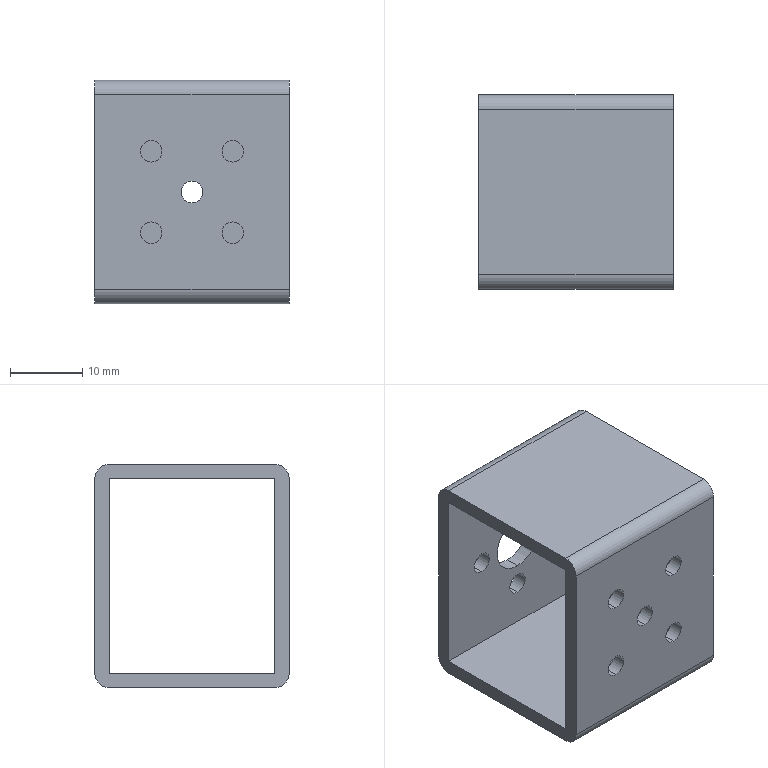Part | SolidWorks | features ICE 4, Fillet 2, Extrusion 1 | 1 solid | 34 faces | box 27 x 27 x 31 mm | volume 5512 mm3 | cylinder 24 | plane 10 | commonest cylinder face diameters 3 x18 4 x4 8 x2
STEP:
#1=CARTESIAN_POINT('',(-5.657,-11.5,8.343));
#2=VERTEX_POINT('',#1);
#3=CARTESIAN_POINT('',(-5.657,-11.5,11.343));
#4=VERTEX_POINT('',#3);
#5=CARTESIAN_POINT('',(-5.657,-11.5,9.843));
#6=DIRECTION('',(0.,1.,0.));
#7=DIRECTION('',(1.,0.,0.));
#8=AXIS2_PLACEMENT_3D('',#5,#6,#7);
#9=CIRCLE('',#8,1.5);
#10=EDGE_CURVE('',#2,#4,#9,.T.);
#11=ORIENTED_EDGE('',*,*,#10,.T.);
#12=CARTESIAN_POINT('',(-5.657,-13.5,11.343));
#13=VERTEX_POINT('',#12);
#14=CARTESIAN_POINT('',(-5.657,13.501,11.343));
#15=DIRECTION('',(0.,-1.,0.));
#16=VECTOR('',#15,1000.);
#17=LINE('',#14,#16);
#18=EDGE_CURVE('',#4,#13,#17,.T.);
#19=ORIENTED_EDGE('',*,*,#18,.T.);
#20=CARTESIAN_POINT('',(-5.657,-13.5,8.343));
#21=VERTEX_POINT('',#20);
#22=CARTESIAN_POINT('',(-5.657,-13.5,9.843));
#23=DIRECTION('',(0.,-1.,0.));
#24=DIRECTION('',(0.,0.,-1.));
#25=AXIS2_PLACEMENT_3D('',#22,#23,#24);
#26=CIRCLE('',#25,1.5);
#27=EDGE_CURVE('',#13,#21,#26,.T.);
#28=ORIENTED_EDGE('',*,*,#27,.T.);
#29=CARTESIAN_POINT('',(-5.657,13.501,8.343));
#30=DIRECTION('',(0.,-1.,0.));
#31=VECTOR('',#30,1000.);
#32=LINE('',#29,#31);
#33=EDGE_CURVE('',#2,#21,#32,.T.);
#34=ORIENTED_EDGE('',*,*,#33,.F.);
#35=EDGE_LOOP('',(#11,#19,#28,#34));
#36=FACE_OUTER_BOUND('',#35,.T.);
#37=CARTESIAN_POINT('',(-5.657,13.501,9.843));
#38=DIRECTION('',(0.,-1.,0.));
#39=DIRECTION('',(0.,0.,-1.));
#40=AXIS2_PLACEMENT_3D('',#37,#38,#39);
#41=CYLINDRICAL_SURFACE('',#40,1.5);
#42=ADVANCED_FACE('',(#36),#41,.F.);
#43=CARTESIAN_POINT('',(5.657,-11.5,8.343));
#44=VERTEX_POINT('',#43);
#45=CARTESIAN_POINT('',(5.657,-11.5,11.343));
#46=VERTEX_POINT('',#45);
#47=CARTESIAN_POINT('',(5.657,-11.5,9.843));
#48=DIRECTION('',(0.,1.,0.));
#49=DIRECTION('',(1.,0.,0.));
#50=AXIS2_PLACEMENT_3D('',#47,#48,#49);
#51=CIRCLE('',#50,1.5);
#52=EDGE_CURVE('',#44,#46,#51,.T.);
#53=ORIENTED_EDGE('',*,*,#52,.T.);
#54=CARTESIAN_POINT('',(5.657,-13.5,11.343));
#55=VERTEX_POINT('',#54);
#56=CARTESIAN_POINT('',(5.657,13.501,11.343));
#57=DIRECTION('',(0.,-1.,0.));
#58=VECTOR('',#57,1000.);
#59=LINE('',#56,#58);
#60=EDGE_CURVE('',#46,#55,#59,.T.);
#61=ORIENTED_EDGE('',*,*,#60,.T.);
#62=CARTESIAN_POINT('',(5.657,-13.5,8.343));
#63=VERTEX_POINT('',#62);
#64=CARTESIAN_POINT('',(5.657,-13.5,9.843));
#65=DIRECTION('',(0.,-1.,0.));
#66=DIRECTION('',(0.,0.,-1.));
#67=AXIS2_PLACEMENT_3D('',#64,#65,#66);
#68=CIRCLE('',#67,1.5);
#69=EDGE_CURVE('',#55,#63,#68,.T.);
#70=ORIENTED_EDGE('',*,*,#69,.T.);
#71=CARTESIAN_POINT('',(5.657,13.501,8.343));
#72=DIRECTION('',(0.,-1.,0.));
#73=VECTOR('',#72,1000.);
#74=LINE('',#71,#73);
#75=EDGE_CURVE('',#44,#63,#74,.T.);
#76=ORIENTED_EDGE('',*,*,#75,.F.);
#77=EDGE_LOOP('',(#53,#61,#70,#76));
#78=FACE_OUTER_BOUND('',#77,.T.);
#79=CARTESIAN_POINT('',(5.657,13.501,9.843));
#80=DIRECTION('',(0.,-1.,0.));
#81=DIRECTION('',(0.,0.,-1.));
#82=AXIS2_PLACEMENT_3D('',#79,#80,#81);
#83=CYLINDRICAL_SURFACE('',#82,1.5);
#84=ADVANCED_FACE('',(#78),#83,.F.);
#85=CARTESIAN_POINT('',(5.657,-11.5,19.657));
#86=VERTEX_POINT('',#85);
#87=CARTESIAN_POINT('',(5.657,-11.5,22.657));
#88=VERTEX_POINT('',#87);
#89=CARTESIAN_POINT('',(5.657,-11.5,21.157));
#90=DIRECTION('',(0.,1.,0.));
#91=DIRECTION('',(1.,0.,0.));
#92=AXIS2_PLACEMENT_3D('',#89,#90,#91);
#93=CIRCLE('',#92,1.5);
#94=EDGE_CURVE('',#86,#88,#93,.T.);
#95=ORIENTED_EDGE('',*,*,#94,.T.);
#96=CARTESIAN_POINT('',(5.657,-13.5,22.657));
#97=VERTEX_POINT('',#96);
#98=CARTESIAN_POINT('',(5.657,13.501,22.657));
#99=DIRECTION('',(0.,-1.,0.));
#100=VECTOR('',#99,1000.);
#101=LINE('',#98,#100);
#102=EDGE_CURVE('',#88,#97,#101,.T.);
#103=ORIENTED_EDGE('',*,*,#102,.T.);
#104=CARTESIAN_POINT('',(5.657,-13.5,19.657));
#105=VERTEX_POINT('',#104);
#106=CARTESIAN_POINT('',(5.657,-13.5,21.157));
#107=DIRECTION('',(0.,-1.,0.));
#108=DIRECTION('',(0.,0.,-1.));
#109=AXIS2_PLACEMENT_3D('',#106,#107,#108);
#110=CIRCLE('',#109,1.5);
#111=EDGE_CURVE('',#97,#105,#110,.T.);
#112=ORIENTED_EDGE('',*,*,#111,.T.);
#113=CARTESIAN_POINT('',(5.657,13.501,19.657));
#114=DIRECTION('',(0.,-1.,0.));
#115=VECTOR('',#114,1000.);
#116=LINE('',#113,#115);
#117=EDGE_CURVE('',#86,#105,#116,.T.);
#118=ORIENTED_EDGE('',*,*,#117,.F.);
#119=EDGE_LOOP('',(#95,#103,#112,#118));
#120=FACE_OUTER_BOUND('',#119,.T.);
#121=CARTESIAN_POINT('',(5.657,13.501,21.157));
#122=DIRECTION('',(0.,-1.,0.));
#123=DIRECTION('',(0.,0.,-1.));
#124=AXIS2_PLACEMENT_3D('',#121,#122,#123);
#125=CYLINDRICAL_SURFACE('',#124,1.5);
#126=ADVANCED_FACE('',(#120),#125,.F.);
#127=CARTESIAN_POINT('',(-5.657,-11.5,19.657));
#128=VERTEX_POINT('',#127);
#129=CARTESIAN_POINT('',(-5.657,-11.5,22.657));
#130=VERTEX_POINT('',#129);
#131=CARTESIAN_POINT('',(-5.657,-11.5,21.157));
#132=DIRECTION('',(0.,1.,0.));
#133=DIRECTION('',(1.,0.,0.));
#134=AXIS2_PLACEMENT_3D('',#131,#132,#133);
#135=CIRCLE('',#134,1.5);
#136=EDGE_CURVE('',#128,#130,#135,.T.);
#137=ORIENTED_EDGE('',*,*,#136,.T.);
#138=CARTESIAN_POINT('',(-5.657,-13.5,22.657));
#139=VERTEX_POINT('',#138);
#140=CARTESIAN_POINT('',(-5.657,13.501,22.657));
#141=DIRECTION('',(0.,-1.,0.));
#142=VECTOR('',#141,1000.);
#143=LINE('',#140,#142);
#144=EDGE_CURVE('',#130,#139,#143,.T.);
#145=ORIENTED_EDGE('',*,*,#144,.T.);
#146=CARTESIAN_POINT('',(-5.657,-13.5,19.657));
#147=VERTEX_POINT('',#146);
#148=CARTESIAN_POINT('',(-5.657,-13.5,21.157));
#149=DIRECTION('',(0.,-1.,0.));
#150=DIRECTION('',(0.,0.,-1.));
#151=AXIS2_PLACEMENT_3D('',#148,#149,#150);
#152=CIRCLE('',#151,1.5);
#153=EDGE_CURVE('',#139,#147,#152,.T.);
#154=ORIENTED_EDGE('',*,*,#153,.T.);
#155=CARTESIAN_POINT('',(-5.657,13.501,19.657));
#156=DIRECTION('',(0.,-1.,0.));
#157=VECTOR('',#156,1000.);
#158=LINE('',#155,#157);
#159=EDGE_CURVE('',#128,#147,#158,.T.);
#160=ORIENTED_EDGE('',*,*,#159,.F.);
#161=EDGE_LOOP('',(#137,#145,#154,#160));
#162=FACE_OUTER_BOUND('',#161,.T.);
#163=CARTESIAN_POINT('',(-5.657,13.501,21.157));
#164=DIRECTION('',(0.,-1.,0.));
#165=DIRECTION('',(0.,0.,-1.));
#166=AXIS2_PLACEMENT_3D('',#163,#164,#165);
#167=CYLINDRICAL_SURFACE('',#166,1.5);
#168=ADVANCED_FACE('',(#162),#167,.F.);
#169=CARTESIAN_POINT('',(0.,-11.5,14.));
#170=VERTEX_POINT('',#169);
#171=CARTESIAN_POINT('',(0.,-11.5,17.));
#172=VERTEX_POINT('',#171);
#173=CARTESIAN_POINT('',(0.,-11.5,15.5));
#174=DIRECTION('',(0.,1.,0.));
#175=DIRECTION('',(1.,0.,0.));
#176=AXIS2_PLACEMENT_3D('',#173,#174,#175);
#177=CIRCLE('',#176,1.5);
#178=EDGE_CURVE('',#170,#172,#177,.T.);
#179=ORIENTED_EDGE('',*,*,#178,.T.);
#180=CARTESIAN_POINT('',(0.,-13.5,17.));
#181=VERTEX_POINT('',#180);
#182=CARTESIAN_POINT('',(0.,13.501,17.));
#183=DIRECTION('',(0.,-1.,0.));
#184=VECTOR('',#183,1000.);
#185=LINE('',#182,#184);
#186=EDGE_CURVE('',#172,#181,#185,.T.);
#187=ORIENTED_EDGE('',*,*,#186,.T.);
#188=CARTESIAN_POINT('',(0.,-13.5,14.));
#189=VERTEX_POINT('',#188);
#190=CARTESIAN_POINT('',(0.,-13.5,15.5));
#191=DIRECTION('',(0.,-1.,0.));
#192=DIRECTION('',(0.,0.,-1.));
#193=AXIS2_PLACEMENT_3D('',#190,#191,#192);
#194=CIRCLE('',#193,1.5);
#195=EDGE_CURVE('',#181,#189,#194,.T.);
#196=ORIENTED_EDGE('',*,*,#195,.T.);
#197=CARTESIAN_POINT('',(0.,13.501,14.));
#198=DIRECTION('',(0.,-1.,0.));
#199=VECTOR('',#198,1000.);
#200=LINE('',#197,#199);
#201=EDGE_CURVE('',#170,#189,#200,.T.);
#202=ORIENTED_EDGE('',*,*,#201,.F.);
#203=EDGE_LOOP('',(#179,#187,#196,#202));
#204=FACE_OUTER_BOUND('',#203,.T.);
#205=CARTESIAN_POINT('',(0.,13.501,15.5));
#206=DIRECTION('',(0.,-1.,0.));
#207=DIRECTION('',(0.,0.,-1.));
#208=AXIS2_PLACEMENT_3D('',#205,#206,#207);
#209=CYLINDRICAL_SURFACE('',#208,1.5);
#210=ADVANCED_FACE('',(#204),#209,.F.);
#211=CARTESIAN_POINT('',(0.,11.5,10.));
#212=VERTEX_POINT('',#211);
#213=CARTESIAN_POINT('',(0.,11.5,7.));
#214=VERTEX_POINT('',#213);
#215=CARTESIAN_POINT('',(0.,11.5,8.5));
#216=DIRECTION('',(0.,-1.,0.));
#217=DIRECTION('',(-1.,0.,0.));
#218=AXIS2_PLACEMENT_3D('',#215,#216,#217);
#219=CIRCLE('',#218,1.5);
#220=EDGE_CURVE('',#212,#214,#219,.T.);
#221=ORIENTED_EDGE('',*,*,#220,.T.);
#222=CARTESIAN_POINT('',(0.,13.5,7.));
#223=VERTEX_POINT('',#222);
#224=CARTESIAN_POINT('',(0.,-13.501,7.));
#225=DIRECTION('',(0.,1.,0.));
#226=VECTOR('',#225,1000.);
#227=LINE('',#224,#226);
#228=EDGE_CURVE('',#214,#223,#227,.T.);
#229=ORIENTED_EDGE('',*,*,#228,.T.);
#230=CARTESIAN_POINT('',(0.,13.5,10.));
#231=VERTEX_POINT('',#230);
#232=CARTESIAN_POINT('',(0.,13.5,8.5));
#233=DIRECTION('',(0.,1.,0.));
#234=DIRECTION('',(0.,0.,1.));
#235=AXIS2_PLACEMENT_3D('',#232,#233,#234);
#236=CIRCLE('',#235,1.5);
#237=EDGE_CURVE('',#223,#231,#236,.T.);
#238=ORIENTED_EDGE('',*,*,#237,.T.);
#239=CARTESIAN_POINT('',(0.,-13.501,10.));
#240=DIRECTION('',(0.,1.,0.));
#241=VECTOR('',#240,1000.);
#242=LINE('',#239,#241);
#243=EDGE_CURVE('',#212,#231,#242,.T.);
#244=ORIENTED_EDGE('',*,*,#243,.F.);
#245=EDGE_LOOP('',(#221,#229,#238,#244));
#246=FACE_OUTER_BOUND('',#245,.T.);
#247=CARTESIAN_POINT('',(0.,-13.501,8.5));
#248=DIRECTION('',(0.,1.,0.));
#249=DIRECTION('',(0.,0.,1.));
#250=AXIS2_PLACEMENT_3D('',#247,#248,#249);
#251=CYLINDRICAL_SURFACE('',#250,1.5);
#252=ADVANCED_FACE('',(#246),#251,.F.);
#253=CARTESIAN_POINT('',(7.,11.5,17.));
#254=VERTEX_POINT('',#253);
#255=CARTESIAN_POINT('',(7.,11.5,14.));
#256=VERTEX_POINT('',#255);
#257=CARTESIAN_POINT('',(7.,11.5,15.5));
#258=DIRECTION('',(0.,-1.,0.));
#259=DIRECTION('',(-1.,0.,0.));
#260=AXIS2_PLACEMENT_3D('',#257,#258,#259);
#261=CIRCLE('',#260,1.5);
#262=EDGE_CURVE('',#254,#256,#261,.T.);
#263=ORIENTED_EDGE('',*,*,#262,.T.);
#264=CARTESIAN_POINT('',(7.,13.5,14.));
#265=VERTEX_POINT('',#264);
#266=CARTESIAN_POINT('',(7.,-13.501,14.));
#267=DIRECTION('',(0.,1.,0.));
#268=VECTOR('',#267,1000.);
#269=LINE('',#266,#268);
#270=EDGE_CURVE('',#256,#265,#269,.T.);
#271=ORIENTED_EDGE('',*,*,#270,.T.);
#272=CARTESIAN_POINT('',(7.,13.5,17.));
#273=VERTEX_POINT('',#272);
#274=CARTESIAN_POINT('',(7.,13.5,15.5));
#275=DIRECTION('',(0.,1.,0.));
#276=DIRECTION('',(0.,0.,1.));
#277=AXIS2_PLACEMENT_3D('',#274,#275,#276);
#278=CIRCLE('',#277,1.5);
#279=EDGE_CURVE('',#265,#273,#278,.T.);
#280=ORIENTED_EDGE('',*,*,#279,.T.);
#281=CARTESIAN_POINT('',(7.,-13.501,17.));
#282=DIRECTION('',(0.,1.,0.));
#283=VECTOR('',#282,1000.);
#284=LINE('',#281,#283);
#285=EDGE_CURVE('',#254,#273,#284,.T.);
#286=ORIENTED_EDGE('',*,*,#285,.F.);
#287=EDGE_LOOP('',(#263,#271,#280,#286));
#288=FACE_OUTER_BOUND('',#287,.T.);
#289=CARTESIAN_POINT('',(7.,-13.501,15.5));
#290=DIRECTION('',(0.,1.,0.));
#291=DIRECTION('',(0.,0.,1.));
#292=AXIS2_PLACEMENT_3D('',#289,#290,#291);
#293=CYLINDRICAL_SURFACE('',#292,1.5);
#294=ADVANCED_FACE('',(#288),#293,.F.);
#295=CARTESIAN_POINT('',(0.,11.5,24.));
#296=VERTEX_POINT('',#295);
#297=CARTESIAN_POINT('',(0.,11.5,21.));
#298=VERTEX_POINT('',#297);
#299=CARTESIAN_POINT('',(0.,11.5,22.5));
#300=DIRECTION('',(0.,-1.,0.));
#301=DIRECTION('',(-1.,0.,0.));
#302=AXIS2_PLACEMENT_3D('',#299,#300,#301);
#303=CIRCLE('',#302,1.5);
#304=EDGE_CURVE('',#296,#298,#303,.T.);
#305=ORIENTED_EDGE('',*,*,#304,.T.);
#306=CARTESIAN_POINT('',(0.,13.5,21.));
#307=VERTEX_POINT('',#306);
#308=CARTESIAN_POINT('',(0.,-13.501,21.));
#309=DIRECTION('',(0.,1.,0.));
#310=VECTOR('',#309,1000.);
#311=LINE('',#308,#310);
#312=EDGE_CURVE('',#298,#307,#311,.T.);
#313=ORIENTED_EDGE('',*,*,#312,.T.);
#314=CARTESIAN_POINT('',(0.,13.5,24.));
#315=VERTEX_POINT('',#314);
#316=CARTESIAN_POINT('',(0.,13.5,22.5));
#317=DIRECTION('',(0.,1.,0.));
#318=DIRECTION('',(0.,0.,1.));
#319=AXIS2_PLACEMENT_3D('',#316,#317,#318);
#320=CIRCLE('',#319,1.5);
#321=EDGE_CURVE('',#307,#315,#320,.T.);
#322=ORIENTED_EDGE('',*,*,#321,.T.);
#323=CARTESIAN_POINT('',(0.,-13.501,24.));
#324=DIRECTION('',(0.,1.,0.));
#325=VECTOR('',#324,1000.);
#326=LINE('',#323,#325);
#327=EDGE_CURVE('',#296,#315,#326,.T.);
#328=ORIENTED_EDGE('',*,*,#327,.F.);
#329=EDGE_LOOP('',(#305,#313,#322,#328));
#330=FACE_OUTER_BOUND('',#329,.T.);
#331=CARTESIAN_POINT('',(0.,-13.501,22.5));
#332=DIRECTION('',(0.,1.,0.));
#333=DIRECTION('',(0.,0.,1.));
#334=AXIS2_PLACEMENT_3D('',#331,#332,#333);
#335=CYLINDRICAL_SURFACE('',#334,1.5);
#336=ADVANCED_FACE('',(#330),#335,.F.);
#337=CARTESIAN_POINT('',(-7.,11.5,17.));
#338=VERTEX_POINT('',#337);
#339=CARTESIAN_POINT('',(-7.,11.5,14.));
#340=VERTEX_POINT('',#339);
#341=CARTESIAN_POINT('',(-7.,11.5,15.5));
#342=DIRECTION('',(0.,-1.,0.));
#343=DIRECTION('',(-1.,0.,0.));
#344=AXIS2_PLACEMENT_3D('',#341,#342,#343);
#345=CIRCLE('',#344,1.5);
#346=EDGE_CURVE('',#338,#340,#345,.T.);
#347=ORIENTED_EDGE('',*,*,#346,.T.);
#348=CARTESIAN_POINT('',(-7.,13.5,14.));
#349=VERTEX_POINT('',#348);
#350=CARTESIAN_POINT('',(-7.,-13.501,14.));
#351=DIRECTION('',(0.,1.,0.));
#352=VECTOR('',#351,1000.);
#353=LINE('',#350,#352);
#354=EDGE_CURVE('',#340,#349,#353,.T.);
#355=ORIENTED_EDGE('',*,*,#354,.T.);
#356=CARTESIAN_POINT('',(-7.,13.5,17.));
#357=VERTEX_POINT('',#356);
#358=CARTESIAN_POINT('',(-7.,13.5,15.5));
#359=DIRECTION('',(0.,1.,0.));
#360=DIRECTION('',(0.,0.,1.));
#361=AXIS2_PLACEMENT_3D('',#358,#359,#360);
#362=CIRCLE('',#361,1.5);
#363=EDGE_CURVE('',#349,#357,#362,.T.);
#364=ORIENTED_EDGE('',*,*,#363,.T.);
#365=CARTESIAN_POINT('',(-7.,-13.501,17.));
#366=DIRECTION('',(0.,1.,0.));
#367=VECTOR('',#366,1000.);
#368=LINE('',#365,#367);
#369=EDGE_CURVE('',#338,#357,#368,.T.);
#370=ORIENTED_EDGE('',*,*,#369,.F.);
#371=EDGE_LOOP('',(#347,#355,#364,#370));
#372=FACE_OUTER_BOUND('',#371,.T.);
#373=CARTESIAN_POINT('',(-7.,-13.501,15.5));
#374=DIRECTION('',(0.,1.,0.));
#375=DIRECTION('',(0.,0.,1.));
#376=AXIS2_PLACEMENT_3D('',#373,#374,#375);
#377=CYLINDRICAL_SURFACE('',#376,1.5);
#378=ADVANCED_FACE('',(#372),#377,.F.);
#379=CARTESIAN_POINT('',(0.,11.5,19.5));
#380=VERTEX_POINT('',#379);
#381=CARTESIAN_POINT('',(0.,11.5,11.5));
#382=VERTEX_POINT('',#381);
#383=CARTESIAN_POINT('',(0.,11.5,15.5));
#384=DIRECTION('',(0.,-1.,0.));
#385=DIRECTION('',(-1.,0.,0.));
#386=AXIS2_PLACEMENT_3D('',#383,#384,#385);
#387=CIRCLE('',#386,4.);
#388=EDGE_CURVE('',#380,#382,#387,.T.);
#389=ORIENTED_EDGE('',*,*,#388,.T.);
#390=CARTESIAN_POINT('',(0.,13.5,11.5));
#391=VERTEX_POINT('',#390);
#392=CARTESIAN_POINT('',(0.,-13.501,11.5));
#393=DIRECTION('',(0.,1.,0.));
#394=VECTOR('',#393,1000.);
#395=LINE('',#392,#394);
#396=EDGE_CURVE('',#382,#391,#395,.T.);
#397=ORIENTED_EDGE('',*,*,#396,.T.);
#398=CARTESIAN_POINT('',(0.,13.5,19.5));
#399=VERTEX_POINT('',#398);
#400=CARTESIAN_POINT('',(0.,13.5,15.5));
#401=DIRECTION('',(0.,1.,0.));
#402=DIRECTION('',(0.,0.,1.));
#403=AXIS2_PLACEMENT_3D('',#400,#401,#402);
#404=CIRCLE('',#403,4.);
#405=EDGE_CURVE('',#391,#399,#404,.T.);
#406=ORIENTED_EDGE('',*,*,#405,.T.);
#407=CARTESIAN_POINT('',(0.,-13.501,19.5));
#408=DIRECTION('',(0.,1.,0.));
#409=VECTOR('',#408,1000.);
#410=LINE('',#407,#409);
#411=EDGE_CURVE('',#380,#399,#410,.T.);
#412=ORIENTED_EDGE('',*,*,#411,.F.);
#413=EDGE_LOOP('',(#389,#397,#406,#412));
#414=FACE_OUTER_BOUND('',#413,.T.);
#415=CARTESIAN_POINT('',(0.,-13.501,15.5));
#416=DIRECTION('',(0.,1.,0.));
#417=DIRECTION('',(0.,0.,1.));
#418=AXIS2_PLACEMENT_3D('',#415,#416,#417);
#419=CYLINDRICAL_SURFACE('',#418,4.);
#420=ADVANCED_FACE('',(#414),#419,.F.);
#421=CARTESIAN_POINT('',(13.5,11.5,31.));
#422=VERTEX_POINT('',#421);
#423=CARTESIAN_POINT('',(13.5,-11.5,31.));
#424=VERTEX_POINT('',#423);
#425=CARTESIAN_POINT('',(13.5,40.574,31.));
#426=DIRECTION('',(0.,-1.,0.));
#427=VECTOR('',#426,1000.);
#428=LINE('',#425,#427);
#429=EDGE_CURVE('',#422,#424,#428,.T.);
#430=ORIENTED_EDGE('',*,*,#429,.T.);
#431=CARTESIAN_POINT('',(13.5,-13.5,29.));
#432=VERTEX_POINT('',#431);
#433=CARTESIAN_POINT('',(13.5,-11.5,29.));
#434=DIRECTION('',(1.,0.,0.));
#435=DIRECTION('',(0.,-1.,0.));
#436=AXIS2_PLACEMENT_3D('',#433,#434,#435);
#437=CIRCLE('',#436,2.);
#438=EDGE_CURVE('',#424,#432,#437,.T.);
#439=ORIENTED_EDGE('',*,*,#438,.T.);
#440=CARTESIAN_POINT('',(13.5,-13.5,2.));
#441=VERTEX_POINT('',#440);
#442=CARTESIAN_POINT('',(13.5,-13.5,29.));
#443=DIRECTION('',(0.,0.,-1.));
#444=VECTOR('',#443,1000.);
#445=LINE('',#442,#444);
#446=EDGE_CURVE('',#432,#441,#445,.T.);
#447=ORIENTED_EDGE('',*,*,#446,.T.);
#448=CARTESIAN_POINT('',(13.5,-11.5,0.));
#449=VERTEX_POINT('',#448);
#450=CARTESIAN_POINT('',(13.5,-11.5,2.));
#451=DIRECTION('',(1.,0.,0.));
#452=DIRECTION('',(0.,-1.,0.));
#453=AXIS2_PLACEMENT_3D('',#450,#451,#452);
#454=CIRCLE('',#453,2.);
#455=EDGE_CURVE('',#441,#449,#454,.T.);
#456=ORIENTED_EDGE('',*,*,#455,.T.);
#457=CARTESIAN_POINT('',(13.5,11.5,0.));
#458=VERTEX_POINT('',#457);
#459=CARTESIAN_POINT('',(13.5,13.5,0.));
#460=DIRECTION('',(0.,1.,0.));
#461=VECTOR('',#460,1000.);
#462=LINE('',#459,#461);
#463=EDGE_CURVE('',#449,#458,#462,.T.);
#464=ORIENTED_EDGE('',*,*,#463,.T.);
#465=CARTESIAN_POINT('',(13.5,13.5,2.));
#466=VERTEX_POINT('',#465);
#467=CARTESIAN_POINT('',(13.5,11.5,2.));
#468=DIRECTION('',(1.,0.,0.));
#469=DIRECTION('',(0.,-1.,0.));
#470=AXIS2_PLACEMENT_3D('',#467,#468,#469);
#471=CIRCLE('',#470,2.);
#472=EDGE_CURVE('',#458,#466,#471,.T.);
#473=ORIENTED_EDGE('',*,*,#472,.T.);
#474=CARTESIAN_POINT('',(13.5,13.5,29.));
#475=VERTEX_POINT('',#474);
#476=CARTESIAN_POINT('',(13.5,13.5,29.));
#477=DIRECTION('',(0.,0.,-1.));
#478=VECTOR('',#477,1000.);
#479=LINE('',#476,#478);
#480=EDGE_CURVE('',#475,#466,#479,.T.);
#481=ORIENTED_EDGE('',*,*,#480,.F.);
#482=CARTESIAN_POINT('',(13.5,11.5,29.));
#483=DIRECTION('',(1.,0.,0.));
#484=DIRECTION('',(0.,-1.,0.));
#485=AXIS2_PLACEMENT_3D('',#482,#483,#484);
#486=CIRCLE('',#485,2.);
#487=EDGE_CURVE('',#475,#422,#486,.T.);
#488=ORIENTED_EDGE('',*,*,#487,.T.);
#489=EDGE_LOOP('',(#430,#439,#447,#456,#464,#473,#481,#488));
#490=FACE_OUTER_BOUND('',#489,.T.);
#491=CARTESIAN_POINT('',(13.5,11.5,29.));
#492=VERTEX_POINT('',#491);
#493=CARTESIAN_POINT('',(13.5,-11.5,29.));
#494=VERTEX_POINT('',#493);
#495=CARTESIAN_POINT('',(13.5,40.574,29.));
#496=DIRECTION('',(0.,-1.,0.));
#497=VECTOR('',#496,1000.);
#498=LINE('',#495,#497);
#499=EDGE_CURVE('',#492,#494,#498,.T.);
#500=ORIENTED_EDGE('',*,*,#499,.F.);
#501=CARTESIAN_POINT('',(13.5,11.5,2.));
#502=VERTEX_POINT('',#501);
#503=CARTESIAN_POINT('',(13.5,11.5,29.));
#504=DIRECTION('',(0.,0.,1.));
#505=VECTOR('',#504,1000.);
#506=LINE('',#503,#505);
#507=EDGE_CURVE('',#502,#492,#506,.T.);
#508=ORIENTED_EDGE('',*,*,#507,.F.);
#509=CARTESIAN_POINT('',(13.5,-11.5,2.));
#510=VERTEX_POINT('',#509);
#511=CARTESIAN_POINT('',(13.5,11.5,2.));
#512=DIRECTION('',(0.,1.,0.));
#513=VECTOR('',#512,1000.);
#514=LINE('',#511,#513);
#515=EDGE_CURVE('',#510,#502,#514,.T.);
#516=ORIENTED_EDGE('',*,*,#515,.F.);
#517=CARTESIAN_POINT('',(13.5,-11.5,29.));
#518=DIRECTION('',(0.,0.,-1.));
#519=VECTOR('',#518,1000.);
#520=LINE('',#517,#519);
#521=EDGE_CURVE('',#494,#510,#520,.T.);
#522=ORIENTED_EDGE('',*,*,#521,.F.);
#523=EDGE_LOOP('',(#500,#508,#516,#522));
#524=FACE_BOUND('',#523,.T.);
#525=CARTESIAN_POINT('',(13.5,13.5,29.));
#526=DIRECTION('',(-1.,0.,0.));
#527=DIRECTION('',(0.,-1.,0.));
#528=AXIS2_PLACEMENT_3D('',#525,#526,#527);
#529=PLANE('',#528);
#530=ADVANCED_FACE('',(#490,#524),#529,.F.);
#531=CARTESIAN_POINT('',(0.,13.5,8.5));
#532=DIRECTION('',(0.,1.,0.));
#533=DIRECTION('',(0.,0.,1.));
#534=AXIS2_PLACEMENT_3D('',#531,#532,#533);
#535=CIRCLE('',#534,1.5);
#536=EDGE_CURVE('',#231,#223,#535,.T.);
#537=ORIENTED_EDGE('',*,*,#536,.F.);
#538=ORIENTED_EDGE('',*,*,#237,.F.);
#539=EDGE_LOOP('',(#537,#538));
#540=FACE_BOUND('',#539,.T.);
#541=CARTESIAN_POINT('',(7.,13.5,15.5));
#542=DIRECTION('',(0.,1.,0.));
#543=DIRECTION('',(0.,0.,1.));
#544=AXIS2_PLACEMENT_3D('',#541,#542,#543);
#545=CIRCLE('',#544,1.5);
#546=EDGE_CURVE('',#273,#265,#545,.T.);
#547=ORIENTED_EDGE('',*,*,#546,.F.);
#548=ORIENTED_EDGE('',*,*,#279,.F.);
#549=EDGE_LOOP('',(#547,#548));
#550=FACE_BOUND('',#549,.T.);
#551=CARTESIAN_POINT('',(0.,13.5,22.5));
#552=DIRECTION('',(0.,1.,0.));
#553=DIRECTION('',(0.,0.,1.));
#554=AXIS2_PLACEMENT_3D('',#551,#552,#553);
#555=CIRCLE('',#554,1.5);
#556=EDGE_CURVE('',#315,#307,#555,.T.);
#557=ORIENTED_EDGE('',*,*,#556,.F.);
#558=ORIENTED_EDGE('',*,*,#321,.F.);
#559=EDGE_LOOP('',(#557,#558));
#560=FACE_BOUND('',#559,.T.);
#561=CARTESIAN_POINT('',(-7.,13.5,15.5));
#562=DIRECTION('',(0.,1.,0.));
#563=DIRECTION('',(0.,0.,1.));
#564=AXIS2_PLACEMENT_3D('',#561,#562,#563);
#565=CIRCLE('',#564,1.5);
#566=EDGE_CURVE('',#357,#349,#565,.T.);
#567=ORIENTED_EDGE('',*,*,#566,.F.);
#568=ORIENTED_EDGE('',*,*,#363,.F.);
#569=EDGE_LOOP('',(#567,#568));
#570=FACE_BOUND('',#569,.T.);
#571=CARTESIAN_POINT('',(0.,13.5,15.5));
#572=DIRECTION('',(0.,1.,0.));
#573=DIRECTION('',(0.,0.,1.));
#574=AXIS2_PLACEMENT_3D('',#571,#572,#573);
#575=CIRCLE('',#574,4.);
#576=EDGE_CURVE('',#399,#391,#575,.T.);
#577=ORIENTED_EDGE('',*,*,#576,.F.);
#578=ORIENTED_EDGE('',*,*,#405,.F.);
#579=EDGE_LOOP('',(#577,#578));
#580=FACE_BOUND('',#579,.T.);
#581=CARTESIAN_POINT('',(-13.5,13.5,29.));
#582=VERTEX_POINT('',#581);
#583=CARTESIAN_POINT('',(-13.5,13.5,2.));
#584=VERTEX_POINT('',#583);
#585=CARTESIAN_POINT('',(-13.5,13.5,29.));
#586=DIRECTION('',(0.,0.,-1.));
#587=VECTOR('',#586,1000.);
#588=LINE('',#585,#587);
#589=EDGE_CURVE('',#582,#584,#588,.T.);
#590=ORIENTED_EDGE('',*,*,#589,.F.);
#591=CARTESIAN_POINT('',(13.5,13.5,29.));
#592=DIRECTION('',(1.,0.,0.));
#593=VECTOR('',#592,1000.);
#594=LINE('',#591,#593);
#595=EDGE_CURVE('',#582,#475,#594,.T.);
#596=ORIENTED_EDGE('',*,*,#595,.T.);
#597=ORIENTED_EDGE('',*,*,#480,.T.);
#598=CARTESIAN_POINT('',(-13.5,13.5,2.));
#599=DIRECTION('',(-1.,0.,0.));
#600=VECTOR('',#599,1000.);
#601=LINE('',#598,#600);
#602=EDGE_CURVE('',#466,#584,#601,.T.);
#603=ORIENTED_EDGE('',*,*,#602,.T.);
#604=EDGE_LOOP('',(#590,#596,#597,#603));
#605=FACE_OUTER_BOUND('',#604,.T.);
#606=CARTESIAN_POINT('',(-13.5,13.5,29.));
#607=DIRECTION('',(0.,-1.,0.));
#608=DIRECTION('',(0.,0.,-1.));
#609=AXIS2_PLACEMENT_3D('',#606,#607,#608);
#610=PLANE('',#609);
#611=ADVANCED_FACE('',(#540,#550,#560,#570,#580,#605),#610,.F.);
#612=CARTESIAN_POINT('',(-13.5,11.5,2.));
#613=VERTEX_POINT('',#612);
#614=CARTESIAN_POINT('',(-13.5,11.5,29.));
#615=VERTEX_POINT('',#614);
#616=CARTESIAN_POINT('',(-13.5,11.5,29.));
#617=DIRECTION('',(0.,0.,1.));
#618=VECTOR('',#617,1000.);
#619=LINE('',#616,#618);
#620=EDGE_CURVE('',#613,#615,#619,.T.);
#621=ORIENTED_EDGE('',*,*,#620,.T.);
#622=CARTESIAN_POINT('',(-13.5,-11.5,29.));
#623=VERTEX_POINT('',#622);
#624=CARTESIAN_POINT('',(-13.5,40.574,29.));
#625=DIRECTION('',(0.,-1.,0.));
#626=VECTOR('',#625,1000.);
#627=LINE('',#624,#626);
#628=EDGE_CURVE('',#615,#623,#627,.T.);
#629=ORIENTED_EDGE('',*,*,#628,.T.);
#630=CARTESIAN_POINT('',(-13.5,-11.5,2.));
#631=VERTEX_POINT('',#630);
#632=CARTESIAN_POINT('',(-13.5,-11.5,29.));
#633=DIRECTION('',(0.,0.,-1.));
#634=VECTOR('',#633,1000.);
#635=LINE('',#632,#634);
#636=EDGE_CURVE('',#623,#631,#635,.T.);
#637=ORIENTED_EDGE('',*,*,#636,.T.);
#638=CARTESIAN_POINT('',(-13.5,11.5,2.));
#639=DIRECTION('',(0.,1.,0.));
#640=VECTOR('',#639,1000.);
#641=LINE('',#638,#640);
#642=EDGE_CURVE('',#631,#613,#641,.T.);
#643=ORIENTED_EDGE('',*,*,#642,.T.);
#644=EDGE_LOOP('',(#621,#629,#637,#643));
#645=FACE_BOUND('',#644,.T.);
#646=CARTESIAN_POINT('',(-13.5,-13.5,29.));
#647=VERTEX_POINT('',#646);
#648=CARTESIAN_POINT('',(-13.5,-13.5,2.));
#649=VERTEX_POINT('',#648);
#650=CARTESIAN_POINT('',(-13.5,-13.5,29.));
#651=DIRECTION('',(0.,0.,-1.));
#652=VECTOR('',#651,1000.);
#653=LINE('',#650,#652);
#654=EDGE_CURVE('',#647,#649,#653,.T.);
#655=ORIENTED_EDGE('',*,*,#654,.F.);
#656=CARTESIAN_POINT('',(-13.5,-11.5,31.));
#657=VERTEX_POINT('',#656);
#658=CARTESIAN_POINT('',(-13.5,-11.5,29.));
#659=DIRECTION('',(-1.,0.,0.));
#660=DIRECTION('',(0.,1.,0.));
#661=AXIS2_PLACEMENT_3D('',#658,#659,#660);
#662=CIRCLE('',#661,2.);
#663=EDGE_CURVE('',#647,#657,#662,.T.);
#664=ORIENTED_EDGE('',*,*,#663,.T.);
#665=CARTESIAN_POINT('',(-13.5,11.5,31.));
#666=VERTEX_POINT('',#665);
#667=CARTESIAN_POINT('',(-13.5,40.574,31.));
#668=DIRECTION('',(0.,-1.,0.));
#669=VECTOR('',#668,1000.);
#670=LINE('',#667,#669);
#671=EDGE_CURVE('',#666,#657,#670,.T.);
#672=ORIENTED_EDGE('',*,*,#671,.F.);
#673=CARTESIAN_POINT('',(-13.5,11.5,29.));
#674=DIRECTION('',(-1.,0.,0.));
#675=DIRECTION('',(0.,1.,0.));
#676=AXIS2_PLACEMENT_3D('',#673,#674,#675);
#677=CIRCLE('',#676,2.);
#678=EDGE_CURVE('',#666,#582,#677,.T.);
#679=ORIENTED_EDGE('',*,*,#678,.T.);
#680=ORIENTED_EDGE('',*,*,#589,.T.);
#681=CARTESIAN_POINT('',(-13.5,11.5,0.));
#682=VERTEX_POINT('',#681);
#683=CARTESIAN_POINT('',(-13.5,11.5,2.));
#684=DIRECTION('',(-1.,0.,0.));
#685=DIRECTION('',(0.,1.,0.));
#686=AXIS2_PLACEMENT_3D('',#683,#684,#685);
#687=CIRCLE('',#686,2.);
#688=EDGE_CURVE('',#584,#682,#687,.T.);
#689=ORIENTED_EDGE('',*,*,#688,.T.);
#690=CARTESIAN_POINT('',(-13.5,-11.5,0.));
#691=VERTEX_POINT('',#690);
#692=CARTESIAN_POINT('',(-13.5,13.5,0.));
#693=DIRECTION('',(0.,-1.,0.));
#694=VECTOR('',#693,1000.);
#695=LINE('',#692,#694);
#696=EDGE_CURVE('',#682,#691,#695,.T.);
#697=ORIENTED_EDGE('',*,*,#696,.T.);
#698=CARTESIAN_POINT('',(-13.5,-11.5,2.));
#699=DIRECTION('',(-1.,0.,0.));
#700=DIRECTION('',(0.,1.,0.));
#701=AXIS2_PLACEMENT_3D('',#698,#699,#700);
#702=CIRCLE('',#701,2.);
#703=EDGE_CURVE('',#691,#649,#702,.T.);
#704=ORIENTED_EDGE('',*,*,#703,.T.);
#705=EDGE_LOOP('',(#655,#664,#672,#679,#680,#689,#697,#704));
#706=FACE_OUTER_BOUND('',#705,.T.);
#707=CARTESIAN_POINT('',(-13.5,13.5,29.));
#708=DIRECTION('',(1.,0.,0.));
#709=DIRECTION('',(0.,1.,0.));
#710=AXIS2_PLACEMENT_3D('',#707,#708,#709);
#711=PLANE('',#710);
#712=ADVANCED_FACE('',(#645,#706),#711,.F.);
#713=CARTESIAN_POINT('',(-5.657,-13.5,9.843));
#714=DIRECTION('',(0.,-1.,0.));
#715=DIRECTION('',(0.,0.,-1.));
#716=AXIS2_PLACEMENT_3D('',#713,#714,#715);
#717=CIRCLE('',#716,1.5);
#718=EDGE_CURVE('',#21,#13,#717,.T.);
#719=ORIENTED_EDGE('',*,*,#718,.F.);
#720=ORIENTED_EDGE('',*,*,#27,.F.);
#721=EDGE_LOOP('',(#719,#720));
#722=FACE_BOUND('',#721,.T.);
#723=CARTESIAN_POINT('',(5.657,-13.5,9.843));
#724=DIRECTION('',(0.,-1.,0.));
#725=DIRECTION('',(0.,0.,-1.));
#726=AXIS2_PLACEMENT_3D('',#723,#724,#725);
#727=CIRCLE('',#726,1.5);
#728=EDGE_CURVE('',#63,#55,#727,.T.);
#729=ORIENTED_EDGE('',*,*,#728,.F.);
#730=ORIENTED_EDGE('',*,*,#69,.F.);
#731=EDGE_LOOP('',(#729,#730));
#732=FACE_BOUND('',#731,.T.);
#733=CARTESIAN_POINT('',(5.657,-13.5,21.157));
#734=DIRECTION('',(0.,-1.,0.));
#735=DIRECTION('',(0.,0.,-1.));
#736=AXIS2_PLACEMENT_3D('',#733,#734,#735);
#737=CIRCLE('',#736,1.5);
#738=EDGE_CURVE('',#105,#97,#737,.T.);
#739=ORIENTED_EDGE('',*,*,#738,.F.);
#740=ORIENTED_EDGE('',*,*,#111,.F.);
#741=EDGE_LOOP('',(#739,#740));
#742=FACE_BOUND('',#741,.T.);
#743=CARTESIAN_POINT('',(-5.657,-13.5,21.157));
#744=DIRECTION('',(0.,-1.,0.));
#745=DIRECTION('',(0.,0.,-1.));
#746=AXIS2_PLACEMENT_3D('',#743,#744,#745);
#747=CIRCLE('',#746,1.5);
#748=EDGE_CURVE('',#147,#139,#747,.T.);
#749=ORIENTED_EDGE('',*,*,#748,.F.);
#750=ORIENTED_EDGE('',*,*,#153,.F.);
#751=EDGE_LOOP('',(#749,#750));
#752=FACE_BOUND('',#751,.T.);
#753=CARTESIAN_POINT('',(0.,-13.5,15.5));
#754=DIRECTION('',(0.,-1.,0.));
#755=DIRECTION('',(0.,0.,-1.));
#756=AXIS2_PLACEMENT_3D('',#753,#754,#755);
#757=CIRCLE('',#756,1.5);
#758=EDGE_CURVE('',#189,#181,#757,.T.);
#759=ORIENTED_EDGE('',*,*,#758,.F.);
#760=ORIENTED_EDGE('',*,*,#195,.F.);
#761=EDGE_LOOP('',(#759,#760));
#762=FACE_BOUND('',#761,.T.);
#763=ORIENTED_EDGE('',*,*,#446,.F.);
#764=CARTESIAN_POINT('',(-13.5,-13.5,29.));
#765=DIRECTION('',(-1.,0.,0.));
#766=VECTOR('',#765,1000.);
#767=LINE('',#764,#766);
#768=EDGE_CURVE('',#432,#647,#767,.T.);
#769=ORIENTED_EDGE('',*,*,#768,.T.);
#770=ORIENTED_EDGE('',*,*,#654,.T.);
#771=CARTESIAN_POINT('',(-13.5,-13.5,2.));
#772=DIRECTION('',(1.,0.,0.));
#773=VECTOR('',#772,1000.);
#774=LINE('',#771,#773);
#775=EDGE_CURVE('',#649,#441,#774,.T.);
#776=ORIENTED_EDGE('',*,*,#775,.T.);
#777=EDGE_LOOP('',(#763,#769,#770,#776));
#778=FACE_OUTER_BOUND('',#777,.T.);
#779=CARTESIAN_POINT('',(-13.5,-13.5,29.));
#780=DIRECTION('',(0.,1.,0.));
#781=DIRECTION('',(0.,0.,1.));
#782=AXIS2_PLACEMENT_3D('',#779,#780,#781);
#783=PLANE('',#782);
#784=ADVANCED_FACE('',(#722,#732,#742,#752,#762,#778),#783,.F.);
#785=ORIENTED_EDGE('',*,*,#696,.F.);
#786=CARTESIAN_POINT('',(0.,11.5,0.));
#787=DIRECTION('',(1.,0.,0.));
#788=VECTOR('',#787,1000.);
#789=LINE('',#786,#788);
#790=EDGE_CURVE('',#682,#458,#789,.T.);
#791=ORIENTED_EDGE('',*,*,#790,.T.);
#792=ORIENTED_EDGE('',*,*,#463,.F.);
#793=CARTESIAN_POINT('',(0.,-11.5,0.));
#794=DIRECTION('',(-1.,0.,0.));
#795=VECTOR('',#794,1000.);
#796=LINE('',#793,#795);
#797=EDGE_CURVE('',#449,#691,#796,.T.);
#798=ORIENTED_EDGE('',*,*,#797,.T.);
#799=EDGE_LOOP('',(#785,#791,#792,#798));
#800=FACE_OUTER_BOUND('',#799,.T.);
#801=CARTESIAN_POINT('',(0.,0.,0.));
#802=DIRECTION('',(0.,0.,1.));
#803=DIRECTION('',(1.,0.,0.));
#804=AXIS2_PLACEMENT_3D('',#801,#802,#803);
#805=PLANE('',#804);
#806=ADVANCED_FACE('',(#800),#805,.F.);
#807=ORIENTED_EDGE('',*,*,#220,.F.);
#808=CARTESIAN_POINT('',(0.,11.5,8.5));
#809=DIRECTION('',(0.,-1.,0.));
#810=DIRECTION('',(-1.,0.,0.));
#811=AXIS2_PLACEMENT_3D('',#808,#809,#810);
#812=CIRCLE('',#811,1.5);
#813=EDGE_CURVE('',#214,#212,#812,.T.);
#814=ORIENTED_EDGE('',*,*,#813,.F.);
#815=EDGE_LOOP('',(#807,#814));
#816=FACE_BOUND('',#815,.T.);
#817=ORIENTED_EDGE('',*,*,#262,.F.);
#818=CARTESIAN_POINT('',(7.,11.5,15.5));
#819=DIRECTION('',(0.,-1.,0.));
#820=DIRECTION('',(-1.,0.,0.));
#821=AXIS2_PLACEMENT_3D('',#818,#819,#820);
#822=CIRCLE('',#821,1.5);
#823=EDGE_CURVE('',#256,#254,#822,.T.);
#824=ORIENTED_EDGE('',*,*,#823,.F.);
#825=EDGE_LOOP('',(#817,#824));
#826=FACE_BOUND('',#825,.T.);
#827=ORIENTED_EDGE('',*,*,#304,.F.);
#828=CARTESIAN_POINT('',(0.,11.5,22.5));
#829=DIRECTION('',(0.,-1.,0.));
#830=DIRECTION('',(-1.,0.,0.));
#831=AXIS2_PLACEMENT_3D('',#828,#829,#830);
#832=CIRCLE('',#831,1.5);
#833=EDGE_CURVE('',#298,#296,#832,.T.);
#834=ORIENTED_EDGE('',*,*,#833,.F.);
#835=EDGE_LOOP('',(#827,#834));
#836=FACE_BOUND('',#835,.T.);
#837=ORIENTED_EDGE('',*,*,#346,.F.);
#838=CARTESIAN_POINT('',(-7.,11.5,15.5));
#839=DIRECTION('',(0.,-1.,0.));
#840=DIRECTION('',(-1.,0.,0.));
#841=AXIS2_PLACEMENT_3D('',#838,#839,#840);
#842=CIRCLE('',#841,1.5);
#843=EDGE_CURVE('',#340,#338,#842,.T.);
#844=ORIENTED_EDGE('',*,*,#843,.F.);
#845=EDGE_LOOP('',(#837,#844));
#846=FACE_BOUND('',#845,.T.);
#847=ORIENTED_EDGE('',*,*,#388,.F.);
#848=CARTESIAN_POINT('',(0.,11.5,15.5));
#849=DIRECTION('',(0.,-1.,0.));
#850=DIRECTION('',(-1.,0.,0.));
#851=AXIS2_PLACEMENT_3D('',#848,#849,#850);
#852=CIRCLE('',#851,4.);
#853=EDGE_CURVE('',#382,#380,#852,.T.);
#854=ORIENTED_EDGE('',*,*,#853,.F.);
#855=EDGE_LOOP('',(#847,#854));
#856=FACE_BOUND('',#855,.T.);
#857=ORIENTED_EDGE('',*,*,#507,.T.);
#858=CARTESIAN_POINT('',(-13.5,11.5,29.));
#859=DIRECTION('',(1.,0.,0.));
#860=VECTOR('',#859,1000.);
#861=LINE('',#858,#860);
#862=EDGE_CURVE('',#615,#492,#861,.T.);
#863=ORIENTED_EDGE('',*,*,#862,.F.);
#864=ORIENTED_EDGE('',*,*,#620,.F.);
#865=CARTESIAN_POINT('',(-13.5,11.5,2.));
#866=DIRECTION('',(1.,0.,0.));
#867=VECTOR('',#866,1000.);
#868=LINE('',#865,#867);
#869=EDGE_CURVE('',#613,#502,#868,.T.);
#870=ORIENTED_EDGE('',*,*,#869,.T.);
#871=EDGE_LOOP('',(#857,#863,#864,#870));
#872=FACE_OUTER_BOUND('',#871,.T.);
#873=CARTESIAN_POINT('',(-13.5,11.5,29.));
#874=DIRECTION('',(0.,1.,0.));
#875=DIRECTION('',(-1.,0.,0.));
#876=AXIS2_PLACEMENT_3D('',#873,#874,#875);
#877=PLANE('',#876);
#878=ADVANCED_FACE('',(#816,#826,#836,#846,#856,#872),#877,.F.);
#879=ORIENTED_EDGE('',*,*,#515,.T.);
#880=ORIENTED_EDGE('',*,*,#869,.F.);
#881=ORIENTED_EDGE('',*,*,#642,.F.);
#882=CARTESIAN_POINT('',(-13.5,-11.5,2.));
#883=DIRECTION('',(1.,0.,0.));
#884=VECTOR('',#883,1000.);
#885=LINE('',#882,#884);
#886=EDGE_CURVE('',#631,#510,#885,.T.);
#887=ORIENTED_EDGE('',*,*,#886,.T.);
#888=EDGE_LOOP('',(#879,#880,#881,#887));
#889=FACE_OUTER_BOUND('',#888,.T.);
#890=CARTESIAN_POINT('',(-13.5,11.5,2.));
#891=DIRECTION('',(0.,0.,-1.));
#892=DIRECTION('',(-1.,0.,0.));
#893=AXIS2_PLACEMENT_3D('',#890,#891,#892);
#894=PLANE('',#893);
#895=ADVANCED_FACE('',(#889),#894,.F.);
#896=ORIENTED_EDGE('',*,*,#10,.F.);
#897=CARTESIAN_POINT('',(-5.657,-11.5,9.843));
#898=DIRECTION('',(0.,1.,0.));
#899=DIRECTION('',(1.,0.,0.));
#900=AXIS2_PLACEMENT_3D('',#897,#898,#899);
#901=CIRCLE('',#900,1.5);
#902=EDGE_CURVE('',#4,#2,#901,.T.);
#903=ORIENTED_EDGE('',*,*,#902,.F.);
#904=EDGE_LOOP('',(#896,#903));
#905=FACE_BOUND('',#904,.T.);
#906=ORIENTED_EDGE('',*,*,#52,.F.);
#907=CARTESIAN_POINT('',(5.657,-11.5,9.843));
#908=DIRECTION('',(0.,1.,0.));
#909=DIRECTION('',(1.,0.,0.));
#910=AXIS2_PLACEMENT_3D('',#907,#908,#909);
#911=CIRCLE('',#910,1.5);
#912=EDGE_CURVE('',#46,#44,#911,.T.);
#913=ORIENTED_EDGE('',*,*,#912,.F.);
#914=EDGE_LOOP('',(#906,#913));
#915=FACE_BOUND('',#914,.T.);
#916=ORIENTED_EDGE('',*,*,#94,.F.);
#917=CARTESIAN_POINT('',(5.657,-11.5,21.157));
#918=DIRECTION('',(0.,1.,0.));
#919=DIRECTION('',(1.,0.,0.));
#920=AXIS2_PLACEMENT_3D('',#917,#918,#919);
#921=CIRCLE('',#920,1.5);
#922=EDGE_CURVE('',#88,#86,#921,.T.);
#923=ORIENTED_EDGE('',*,*,#922,.F.);
#924=EDGE_LOOP('',(#916,#923));
#925=FACE_BOUND('',#924,.T.);
#926=ORIENTED_EDGE('',*,*,#136,.F.);
#927=CARTESIAN_POINT('',(-5.657,-11.5,21.157));
#928=DIRECTION('',(0.,1.,0.));
#929=DIRECTION('',(1.,0.,0.));
#930=AXIS2_PLACEMENT_3D('',#927,#928,#929);
#931=CIRCLE('',#930,1.5);
#932=EDGE_CURVE('',#130,#128,#931,.T.);
#933=ORIENTED_EDGE('',*,*,#932,.F.);
#934=EDGE_LOOP('',(#926,#933));
#935=FACE_BOUND('',#934,.T.);
#936=ORIENTED_EDGE('',*,*,#178,.F.);
#937=CARTESIAN_POINT('',(0.,-11.5,15.5));
#938=DIRECTION('',(0.,1.,0.));
#939=DIRECTION('',(1.,0.,0.));
#940=AXIS2_PLACEMENT_3D('',#937,#938,#939);
#941=CIRCLE('',#940,1.5);
#942=EDGE_CURVE('',#172,#170,#941,.T.);
#943=ORIENTED_EDGE('',*,*,#942,.F.);
#944=EDGE_LOOP('',(#936,#943));
#945=FACE_BOUND('',#944,.T.);
#946=ORIENTED_EDGE('',*,*,#521,.T.);
#947=ORIENTED_EDGE('',*,*,#886,.F.);
#948=ORIENTED_EDGE('',*,*,#636,.F.);
#949=CARTESIAN_POINT('',(-13.5,-11.5,29.));
#950=DIRECTION('',(1.,0.,0.));
#951=VECTOR('',#950,1000.);
#952=LINE('',#949,#951);
#953=EDGE_CURVE('',#623,#494,#952,.T.);
#954=ORIENTED_EDGE('',*,*,#953,.T.);
#955=EDGE_LOOP('',(#946,#947,#948,#954));
#956=FACE_OUTER_BOUND('',#955,.T.);
#957=CARTESIAN_POINT('',(-13.5,-11.5,29.));
#958=DIRECTION('',(0.,-1.,0.));
#959=DIRECTION('',(1.,0.,0.));
#960=AXIS2_PLACEMENT_3D('',#957,#958,#959);
#961=PLANE('',#960);
#962=ADVANCED_FACE('',(#905,#915,#925,#935,#945,#956),#961,.F.);
#963=ORIENTED_EDGE('',*,*,#396,.F.);
#964=ORIENTED_EDGE('',*,*,#853,.T.);
#965=ORIENTED_EDGE('',*,*,#411,.T.);
#966=ORIENTED_EDGE('',*,*,#576,.T.);
#967=EDGE_LOOP('',(#963,#964,#965,#966));
#968=FACE_OUTER_BOUND('',#967,.T.);
#969=CARTESIAN_POINT('',(0.,-13.501,15.5));
#970=DIRECTION('',(0.,1.,0.));
#971=DIRECTION('',(0.,0.,1.));
#972=AXIS2_PLACEMENT_3D('',#969,#970,#971);
#973=CYLINDRICAL_SURFACE('',#972,4.);
#974=ADVANCED_FACE('',(#968),#973,.F.);
#975=ORIENTED_EDGE('',*,*,#354,.F.);
#976=ORIENTED_EDGE('',*,*,#843,.T.);
#977=ORIENTED_EDGE('',*,*,#369,.T.);
#978=ORIENTED_EDGE('',*,*,#566,.T.);
#979=EDGE_LOOP('',(#975,#976,#977,#978));
#980=FACE_OUTER_BOUND('',#979,.T.);
#981=CARTESIAN_POINT('',(-7.,-13.501,15.5));
#982=DIRECTION('',(0.,1.,0.));
#983=DIRECTION('',(0.,0.,1.));
#984=AXIS2_PLACEMENT_3D('',#981,#982,#983);
#985=CYLINDRICAL_SURFACE('',#984,1.5);
#986=ADVANCED_FACE('',(#980),#985,.F.);
#987=ORIENTED_EDGE('',*,*,#312,.F.);
#988=ORIENTED_EDGE('',*,*,#833,.T.);
#989=ORIENTED_EDGE('',*,*,#327,.T.);
#990=ORIENTED_EDGE('',*,*,#556,.T.);
#991=EDGE_LOOP('',(#987,#988,#989,#990));
#992=FACE_OUTER_BOUND('',#991,.T.);
#993=CARTESIAN_POINT('',(0.,-13.501,22.5));
#994=DIRECTION('',(0.,1.,0.));
#995=DIRECTION('',(0.,0.,1.));
#996=AXIS2_PLACEMENT_3D('',#993,#994,#995);
#997=CYLINDRICAL_SURFACE('',#996,1.5);
#998=ADVANCED_FACE('',(#992),#997,.F.);
#999=ORIENTED_EDGE('',*,*,#270,.F.);
#1000=ORIENTED_EDGE('',*,*,#823,.T.);
#1001=ORIENTED_EDGE('',*,*,#285,.T.);
#1002=ORIENTED_EDGE('',*,*,#546,.T.);
#1003=EDGE_LOOP('',(#999,#1000,#1001,#1002));
#1004=FACE_OUTER_BOUND('',#1003,.T.);
#1005=CARTESIAN_POINT('',(7.,-13.501,15.5));
#1006=DIRECTION('',(0.,1.,0.));
#1007=DIRECTION('',(0.,0.,1.));
#1008=AXIS2_PLACEMENT_3D('',#1005,#1006,#1007);
#1009=CYLINDRICAL_SURFACE('',#1008,1.5);
#1010=ADVANCED_FACE('',(#1004),#1009,.F.);
#1011=ORIENTED_EDGE('',*,*,#228,.F.);
#1012=ORIENTED_EDGE('',*,*,#813,.T.);
#1013=ORIENTED_EDGE('',*,*,#243,.T.);
#1014=ORIENTED_EDGE('',*,*,#536,.T.);
#1015=EDGE_LOOP('',(#1011,#1012,#1013,#1014));
#1016=FACE_OUTER_BOUND('',#1015,.T.);
#1017=CARTESIAN_POINT('',(0.,-13.501,8.5));
#1018=DIRECTION('',(0.,1.,0.));
#1019=DIRECTION('',(0.,0.,1.));
#1020=AXIS2_PLACEMENT_3D('',#1017,#1018,#1019);
#1021=CYLINDRICAL_SURFACE('',#1020,1.5);
#1022=ADVANCED_FACE('',(#1016),#1021,.F.);
#1023=ORIENTED_EDGE('',*,*,#186,.F.);
#1024=ORIENTED_EDGE('',*,*,#942,.T.);
#1025=ORIENTED_EDGE('',*,*,#201,.T.);
#1026=ORIENTED_EDGE('',*,*,#758,.T.);
#1027=EDGE_LOOP('',(#1023,#1024,#1025,#1026));
#1028=FACE_OUTER_BOUND('',#1027,.T.);
#1029=CARTESIAN_POINT('',(0.,13.501,15.5));
#1030=DIRECTION('',(0.,-1.,0.));
#1031=DIRECTION('',(0.,0.,-1.));
#1032=AXIS2_PLACEMENT_3D('',#1029,#1030,#1031);
#1033=CYLINDRICAL_SURFACE('',#1032,1.5);
#1034=ADVANCED_FACE('',(#1028),#1033,.F.);
#1035=ORIENTED_EDGE('',*,*,#144,.F.);
#1036=ORIENTED_EDGE('',*,*,#932,.T.);
#1037=ORIENTED_EDGE('',*,*,#159,.T.);
#1038=ORIENTED_EDGE('',*,*,#748,.T.);
#1039=EDGE_LOOP('',(#1035,#1036,#1037,#1038));
#1040=FACE_OUTER_BOUND('',#1039,.T.);
#1041=CARTESIAN_POINT('',(-5.657,13.501,21.157));
#1042=DIRECTION('',(0.,-1.,0.));
#1043=DIRECTION('',(0.,0.,-1.));
#1044=AXIS2_PLACEMENT_3D('',#1041,#1042,#1043);
#1045=CYLINDRICAL_SURFACE('',#1044,1.5);
#1046=ADVANCED_FACE('',(#1040),#1045,.F.);
#1047=ORIENTED_EDGE('',*,*,#102,.F.);
#1048=ORIENTED_EDGE('',*,*,#922,.T.);
#1049=ORIENTED_EDGE('',*,*,#117,.T.);
#1050=ORIENTED_EDGE('',*,*,#738,.T.);
#1051=EDGE_LOOP('',(#1047,#1048,#1049,#1050));
#1052=FACE_OUTER_BOUND('',#1051,.T.);
#1053=CARTESIAN_POINT('',(5.657,13.501,21.157));
#1054=DIRECTION('',(0.,-1.,0.));
#1055=DIRECTION('',(0.,0.,-1.));
#1056=AXIS2_PLACEMENT_3D('',#1053,#1054,#1055);
#1057=CYLINDRICAL_SURFACE('',#1056,1.5);
#1058=ADVANCED_FACE('',(#1052),#1057,.F.);
#1059=ORIENTED_EDGE('',*,*,#60,.F.);
#1060=ORIENTED_EDGE('',*,*,#912,.T.);
#1061=ORIENTED_EDGE('',*,*,#75,.T.);
#1062=ORIENTED_EDGE('',*,*,#728,.T.);
#1063=EDGE_LOOP('',(#1059,#1060,#1061,#1062));
#1064=FACE_OUTER_BOUND('',#1063,.T.);
#1065=CARTESIAN_POINT('',(5.657,13.501,9.843));
#1066=DIRECTION('',(0.,-1.,0.));
#1067=DIRECTION('',(0.,0.,-1.));
#1068=AXIS2_PLACEMENT_3D('',#1065,#1066,#1067);
#1069=CYLINDRICAL_SURFACE('',#1068,1.5);
#1070=ADVANCED_FACE('',(#1064),#1069,.F.);
#1071=ORIENTED_EDGE('',*,*,#18,.F.);
#1072=ORIENTED_EDGE('',*,*,#902,.T.);
#1073=ORIENTED_EDGE('',*,*,#33,.T.);
#1074=ORIENTED_EDGE('',*,*,#718,.T.);
#1075=EDGE_LOOP('',(#1071,#1072,#1073,#1074));
#1076=FACE_OUTER_BOUND('',#1075,.T.);
#1077=CARTESIAN_POINT('',(-5.657,13.501,9.843));
#1078=DIRECTION('',(0.,-1.,0.));
#1079=DIRECTION('',(0.,0.,-1.));
#1080=AXIS2_PLACEMENT_3D('',#1077,#1078,#1079);
#1081=CYLINDRICAL_SURFACE('',#1080,1.5);
#1082=ADVANCED_FACE('',(#1076),#1081,.F.);
#1083=ORIENTED_EDGE('',*,*,#472,.F.);
#1084=ORIENTED_EDGE('',*,*,#790,.F.);
#1085=ORIENTED_EDGE('',*,*,#688,.F.);
#1086=ORIENTED_EDGE('',*,*,#602,.F.);
#1087=EDGE_LOOP('',(#1083,#1084,#1085,#1086));
#1088=FACE_OUTER_BOUND('',#1087,.T.);
#1089=CARTESIAN_POINT('',(-13.5,11.5,2.));
#1090=DIRECTION('',(-1.,0.,0.));
#1091=DIRECTION('',(0.,0.,1.));
#1092=AXIS2_PLACEMENT_3D('',#1089,#1090,#1091);
#1093=CYLINDRICAL_SURFACE('',#1092,2.);
#1094=ADVANCED_FACE('',(#1088),#1093,.T.);
#1095=ORIENTED_EDGE('',*,*,#703,.F.);
#1096=ORIENTED_EDGE('',*,*,#797,.F.);
#1097=ORIENTED_EDGE('',*,*,#455,.F.);
#1098=ORIENTED_EDGE('',*,*,#775,.F.);
#1099=EDGE_LOOP('',(#1095,#1096,#1097,#1098));
#1100=FACE_OUTER_BOUND('',#1099,.T.);
#1101=CARTESIAN_POINT('',(-13.5,-11.5,2.));
#1102=DIRECTION('',(1.,0.,0.));
#1103=DIRECTION('',(0.,0.,-1.));
#1104=AXIS2_PLACEMENT_3D('',#1101,#1102,#1103);
#1105=CYLINDRICAL_SURFACE('',#1104,2.);
#1106=ADVANCED_FACE('',(#1100),#1105,.T.);
#1107=ORIENTED_EDGE('',*,*,#862,.T.);
#1108=ORIENTED_EDGE('',*,*,#499,.T.);
#1109=ORIENTED_EDGE('',*,*,#953,.F.);
#1110=ORIENTED_EDGE('',*,*,#628,.F.);
#1111=EDGE_LOOP('',(#1107,#1108,#1109,#1110));
#1112=FACE_OUTER_BOUND('',#1111,.T.);
#1113=CARTESIAN_POINT('',(-13.5,40.574,29.));
#1114=DIRECTION('',(0.,0.,-1.));
#1115=DIRECTION('',(-1.,0.,0.));
#1116=AXIS2_PLACEMENT_3D('',#1113,#1114,#1115);
#1117=PLANE('',#1116);
#1118=ADVANCED_FACE('',(#1112),#1117,.T.);
#1119=ORIENTED_EDGE('',*,*,#671,.T.);
#1120=CARTESIAN_POINT('',(13.5,-11.5,31.));
#1121=DIRECTION('',(1.,0.,0.));
#1122=VECTOR('',#1121,1000.);
#1123=LINE('',#1120,#1122);
#1124=EDGE_CURVE('',#657,#424,#1123,.T.);
#1125=ORIENTED_EDGE('',*,*,#1124,.T.);
#1126=ORIENTED_EDGE('',*,*,#429,.F.);
#1127=CARTESIAN_POINT('',(-13.5,11.5,31.));
#1128=DIRECTION('',(-1.,0.,0.));
#1129=VECTOR('',#1128,1000.);
#1130=LINE('',#1127,#1129);
#1131=EDGE_CURVE('',#422,#666,#1130,.T.);
#1132=ORIENTED_EDGE('',*,*,#1131,.T.);
#1133=EDGE_LOOP('',(#1119,#1125,#1126,#1132));
#1134=FACE_OUTER_BOUND('',#1133,.T.);
#1135=CARTESIAN_POINT('',(-13.5,40.574,31.));
#1136=DIRECTION('',(0.,0.,1.));
#1137=DIRECTION('',(1.,0.,0.));
#1138=AXIS2_PLACEMENT_3D('',#1135,#1136,#1137);
#1139=PLANE('',#1138);
#1140=ADVANCED_FACE('',(#1134),#1139,.T.);
#1141=ORIENTED_EDGE('',*,*,#438,.F.);
#1142=ORIENTED_EDGE('',*,*,#1124,.F.);
#1143=ORIENTED_EDGE('',*,*,#663,.F.);
#1144=ORIENTED_EDGE('',*,*,#768,.F.);
#1145=EDGE_LOOP('',(#1141,#1142,#1143,#1144));
#1146=FACE_OUTER_BOUND('',#1145,.T.);
#1147=CARTESIAN_POINT('',(-13.5,-11.5,29.));
#1148=DIRECTION('',(1.,0.,0.));
#1149=DIRECTION('',(0.,0.,-1.));
#1150=AXIS2_PLACEMENT_3D('',#1147,#1148,#1149);
#1151=CYLINDRICAL_SURFACE('',#1150,2.);
#1152=ADVANCED_FACE('',(#1146),#1151,.T.);
#1153=ORIENTED_EDGE('',*,*,#678,.F.);
#1154=ORIENTED_EDGE('',*,*,#1131,.F.);
#1155=ORIENTED_EDGE('',*,*,#487,.F.);
#1156=ORIENTED_EDGE('',*,*,#595,.F.);
#1157=EDGE_LOOP('',(#1153,#1154,#1155,#1156));
#1158=FACE_OUTER_BOUND('',#1157,.T.);
#1159=CARTESIAN_POINT('',(-13.5,11.5,29.));
#1160=DIRECTION('',(-1.,0.,0.));
#1161=DIRECTION('',(0.,0.,1.));
#1162=AXIS2_PLACEMENT_3D('',#1159,#1160,#1161);
#1163=CYLINDRICAL_SURFACE('',#1162,2.);
#1164=ADVANCED_FACE('',(#1158),#1163,.T.);
#1165=CLOSED_SHELL('',(#42,#84,#126,#168,#210,#252,#294,#336,#378,#420,#530,#611,#712,#784,#806,#878,#895,#962,#974,#986,#998,#1010,#1022,#1034,#1046,#1058,#1070,#1082,#1094,#1106,#1118,#1140,#1152,#1164));
#1166=MANIFOLD_SOLID_BREP('',#1165);
#1167=CARTESIAN_POINT('',(0.,0.,0.));
#1168=DIRECTION('',(0.,0.,1.));
#1169=DIRECTION('',(1.,0.,0.));
#1170=AXIS2_PLACEMENT_3D('',#1167,#1168,#1169);
#1171=(LENGTH_UNIT()NAMED_UNIT(*)SI_UNIT(.MILLI.,.METRE.));
#1172=UNCERTAINTY_MEASURE_WITH_UNIT(LENGTH_MEASURE(0.00001),#1171,'','');
#1173=(NAMED_UNIT(*)PLANE_ANGLE_UNIT()SI_UNIT($,.RADIAN.));
#1174=(NAMED_UNIT(*)SI_UNIT($,.STERADIAN.)SOLID_ANGLE_UNIT());
#1175=(GEOMETRIC_REPRESENTATION_CONTEXT(3)GLOBAL_UNCERTAINTY_ASSIGNED_CONTEXT((#1172))GLOBAL_UNIT_ASSIGNED_CONTEXT((#1171,#1173,#1174))REPRESENTATION_CONTEXT('',''));
#1176=ADVANCED_BREP_SHAPE_REPRESENTATION('',(#1166,#1170),#1175);